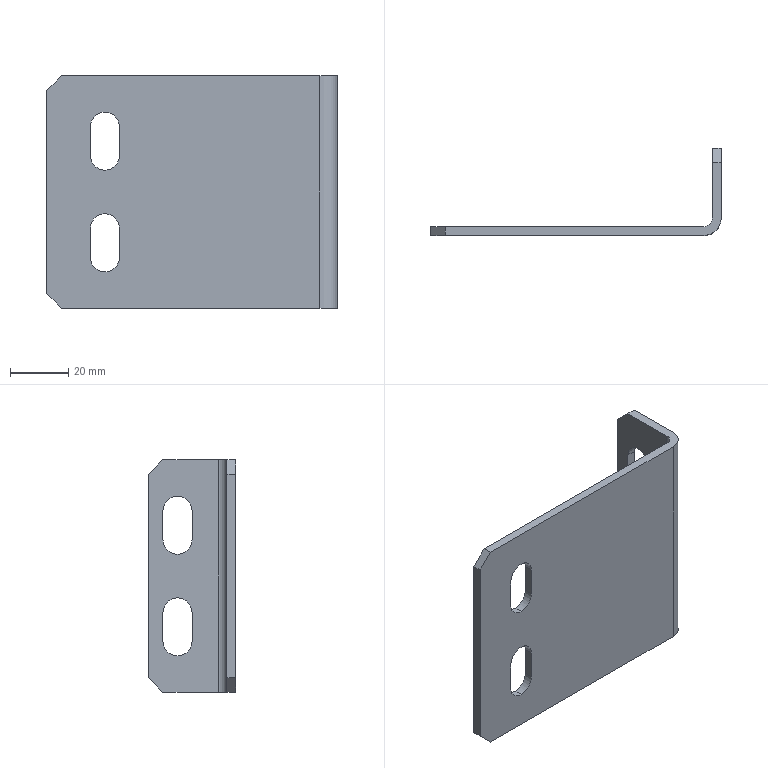Part | STEP file | VD-SYL0380DJ1006_1-9_VD-SYL0380 | 1 solid | 34 faces | box 100 x 30 x 80 mm | volume 27724 mm3 | plane 20 | cylinder 14 | commonest cylinder face diameters 10 x12 6 x1 12 x1
STEP:
#1=CARTESIAN_POINT('',(-75.,3.,-12.5));
#2=VERTEX_POINT('',#1);
#3=CARTESIAN_POINT('',(-85.,3.,-12.5));
#4=VERTEX_POINT('',#3);
#5=CARTESIAN_POINT('',(-80.,3.,-12.5));
#6=DIRECTION('',(0.,-1.,0.));
#7=DIRECTION('',(1.,0.,0.));
#8=AXIS2_PLACEMENT_3D('',#5,#6,#7);
#9=CIRCLE('',#8,5.);
#10=EDGE_CURVE('',#2,#4,#9,.T.);
#11=ORIENTED_EDGE('',*,*,#10,.F.);
#12=CARTESIAN_POINT('',(-75.,0.,-12.5));
#13=VERTEX_POINT('',#12);
#14=CARTESIAN_POINT('',(-75.,3.,-12.5));
#15=DIRECTION('',(0.,-1.,0.));
#16=VECTOR('',#15,1000.);
#17=LINE('',#14,#16);
#18=EDGE_CURVE('',#2,#13,#17,.T.);
#19=ORIENTED_EDGE('',*,*,#18,.T.);
#20=CARTESIAN_POINT('',(-85.,0.,-12.5));
#21=VERTEX_POINT('',#20);
#22=CARTESIAN_POINT('',(-80.,0.,-12.5));
#23=DIRECTION('',(0.,1.,0.));
#24=DIRECTION('',(-1.,0.,0.));
#25=AXIS2_PLACEMENT_3D('',#22,#23,#24);
#26=CIRCLE('',#25,5.);
#27=EDGE_CURVE('',#21,#13,#26,.T.);
#28=ORIENTED_EDGE('',*,*,#27,.F.);
#29=CARTESIAN_POINT('',(-85.,0.,-12.5));
#30=DIRECTION('',(0.,1.,0.));
#31=VECTOR('',#30,1000.);
#32=LINE('',#29,#31);
#33=EDGE_CURVE('',#21,#4,#32,.T.);
#34=ORIENTED_EDGE('',*,*,#33,.T.);
#35=EDGE_LOOP('',(#11,#19,#28,#34));
#36=FACE_OUTER_BOUND('',#35,.T.);
#37=CARTESIAN_POINT('',(-80.,1.5,-12.5));
#38=DIRECTION('',(0.,-1.,0.));
#39=DIRECTION('',(0.,0.,-1.));
#40=AXIS2_PLACEMENT_3D('',#37,#38,#39);
#41=CYLINDRICAL_SURFACE('',#40,5.);
#42=ADVANCED_FACE('',(#36),#41,.F.);
#43=CARTESIAN_POINT('',(-85.,0.,-22.5));
#44=VERTEX_POINT('',#43);
#45=CARTESIAN_POINT('',(-85.,0.,-12.5));
#46=DIRECTION('',(0.,0.,-1.));
#47=VECTOR('',#46,1000.);
#48=LINE('',#45,#47);
#49=EDGE_CURVE('',#21,#44,#48,.T.);
#50=ORIENTED_EDGE('',*,*,#49,.T.);
#51=CARTESIAN_POINT('',(-85.,3.,-22.5));
#52=VERTEX_POINT('',#51);
#53=CARTESIAN_POINT('',(-85.,3.,-22.5));
#54=DIRECTION('',(0.,-1.,0.));
#55=VECTOR('',#54,1000.);
#56=LINE('',#53,#55);
#57=EDGE_CURVE('',#52,#44,#56,.T.);
#58=ORIENTED_EDGE('',*,*,#57,.F.);
#59=CARTESIAN_POINT('',(-85.,3.,-12.5));
#60=DIRECTION('',(0.,0.,-1.));
#61=VECTOR('',#60,1000.);
#62=LINE('',#59,#61);
#63=EDGE_CURVE('',#4,#52,#62,.T.);
#64=ORIENTED_EDGE('',*,*,#63,.F.);
#65=ORIENTED_EDGE('',*,*,#33,.F.);
#66=EDGE_LOOP('',(#50,#58,#64,#65));
#67=FACE_OUTER_BOUND('',#66,.T.);
#68=CARTESIAN_POINT('',(-85.,1.5,-17.5));
#69=DIRECTION('',(1.,0.,0.));
#70=DIRECTION('',(0.,1.,0.));
#71=AXIS2_PLACEMENT_3D('',#68,#69,#70);
#72=PLANE('',#71);
#73=ADVANCED_FACE('',(#67),#72,.T.);
#74=CARTESIAN_POINT('',(-80.,3.,-27.5));
#75=VERTEX_POINT('',#74);
#76=CARTESIAN_POINT('',(-80.,3.,-22.5));
#77=DIRECTION('',(0.,-1.,0.));
#78=DIRECTION('',(-1.,0.,0.));
#79=AXIS2_PLACEMENT_3D('',#76,#77,#78);
#80=CIRCLE('',#79,5.);
#81=EDGE_CURVE('',#52,#75,#80,.T.);
#82=ORIENTED_EDGE('',*,*,#81,.F.);
#83=ORIENTED_EDGE('',*,*,#57,.T.);
#84=CARTESIAN_POINT('',(-80.,0.,-27.5));
#85=VERTEX_POINT('',#84);
#86=CARTESIAN_POINT('',(-80.,0.,-22.5));
#87=DIRECTION('',(0.,1.,0.));
#88=DIRECTION('',(0.,0.,-1.));
#89=AXIS2_PLACEMENT_3D('',#86,#87,#88);
#90=CIRCLE('',#89,5.);
#91=EDGE_CURVE('',#85,#44,#90,.T.);
#92=ORIENTED_EDGE('',*,*,#91,.F.);
#93=CARTESIAN_POINT('',(-80.,0.,-27.5));
#94=DIRECTION('',(0.,1.,0.));
#95=VECTOR('',#94,1000.);
#96=LINE('',#93,#95);
#97=EDGE_CURVE('',#85,#75,#96,.T.);
#98=ORIENTED_EDGE('',*,*,#97,.T.);
#99=EDGE_LOOP('',(#82,#83,#92,#98));
#100=FACE_OUTER_BOUND('',#99,.T.);
#101=CARTESIAN_POINT('',(-80.,1.5,-22.5));
#102=DIRECTION('',(0.,-1.,0.));
#103=DIRECTION('',(0.,0.,-1.));
#104=AXIS2_PLACEMENT_3D('',#101,#102,#103);
#105=CYLINDRICAL_SURFACE('',#104,5.);
#106=ADVANCED_FACE('',(#100),#105,.F.);
#107=ORIENTED_EDGE('',*,*,#97,.F.);
#108=CARTESIAN_POINT('',(-75.,0.,-22.5));
#109=VERTEX_POINT('',#108);
#110=CARTESIAN_POINT('',(-80.,0.,-22.5));
#111=DIRECTION('',(0.,1.,0.));
#112=DIRECTION('',(1.,0.,0.));
#113=AXIS2_PLACEMENT_3D('',#110,#111,#112);
#114=CIRCLE('',#113,5.);
#115=EDGE_CURVE('',#109,#85,#114,.T.);
#116=ORIENTED_EDGE('',*,*,#115,.F.);
#117=CARTESIAN_POINT('',(-75.,3.,-22.5));
#118=VERTEX_POINT('',#117);
#119=CARTESIAN_POINT('',(-75.,0.,-22.5));
#120=DIRECTION('',(0.,1.,0.));
#121=VECTOR('',#120,1000.);
#122=LINE('',#119,#121);
#123=EDGE_CURVE('',#109,#118,#122,.T.);
#124=ORIENTED_EDGE('',*,*,#123,.T.);
#125=CARTESIAN_POINT('',(-80.,3.,-22.5));
#126=DIRECTION('',(0.,-1.,0.));
#127=DIRECTION('',(0.,0.,-1.));
#128=AXIS2_PLACEMENT_3D('',#125,#126,#127);
#129=CIRCLE('',#128,5.);
#130=EDGE_CURVE('',#75,#118,#129,.T.);
#131=ORIENTED_EDGE('',*,*,#130,.F.);
#132=EDGE_LOOP('',(#107,#116,#124,#131));
#133=FACE_OUTER_BOUND('',#132,.T.);
#134=CARTESIAN_POINT('',(-80.,1.5,-22.5));
#135=DIRECTION('',(0.,-1.,0.));
#136=DIRECTION('',(0.,0.,-1.));
#137=AXIS2_PLACEMENT_3D('',#134,#135,#136);
#138=CYLINDRICAL_SURFACE('',#137,5.);
#139=ADVANCED_FACE('',(#133),#138,.F.);
#140=CARTESIAN_POINT('',(-75.,0.,-22.5));
#141=DIRECTION('',(0.,0.,1.));
#142=VECTOR('',#141,1000.);
#143=LINE('',#140,#142);
#144=EDGE_CURVE('',#109,#13,#143,.T.);
#145=ORIENTED_EDGE('',*,*,#144,.T.);
#146=ORIENTED_EDGE('',*,*,#18,.F.);
#147=CARTESIAN_POINT('',(-75.,3.,-22.5));
#148=DIRECTION('',(0.,0.,1.));
#149=VECTOR('',#148,1000.);
#150=LINE('',#147,#149);
#151=EDGE_CURVE('',#118,#2,#150,.T.);
#152=ORIENTED_EDGE('',*,*,#151,.F.);
#153=ORIENTED_EDGE('',*,*,#123,.F.);
#154=EDGE_LOOP('',(#145,#146,#152,#153));
#155=FACE_OUTER_BOUND('',#154,.T.);
#156=CARTESIAN_POINT('',(-75.,1.5,-17.5));
#157=DIRECTION('',(-1.,0.,0.));
#158=DIRECTION('',(0.,0.,1.));
#159=AXIS2_PLACEMENT_3D('',#156,#157,#158);
#160=PLANE('',#159);
#161=ADVANCED_FACE('',(#155),#160,.T.);
#162=CARTESIAN_POINT('',(-85.,0.,22.5));
#163=VERTEX_POINT('',#162);
#164=CARTESIAN_POINT('',(-85.,0.,12.5));
#165=VERTEX_POINT('',#164);
#166=CARTESIAN_POINT('',(-85.,0.,22.5));
#167=DIRECTION('',(0.,0.,-1.));
#168=VECTOR('',#167,1000.);
#169=LINE('',#166,#168);
#170=EDGE_CURVE('',#163,#165,#169,.T.);
#171=ORIENTED_EDGE('',*,*,#170,.T.);
#172=CARTESIAN_POINT('',(-85.,3.,12.5));
#173=VERTEX_POINT('',#172);
#174=CARTESIAN_POINT('',(-85.,3.,12.5));
#175=DIRECTION('',(0.,-1.,0.));
#176=VECTOR('',#175,1000.);
#177=LINE('',#174,#176);
#178=EDGE_CURVE('',#173,#165,#177,.T.);
#179=ORIENTED_EDGE('',*,*,#178,.F.);
#180=CARTESIAN_POINT('',(-85.,3.,22.5));
#181=VERTEX_POINT('',#180);
#182=CARTESIAN_POINT('',(-85.,3.,22.5));
#183=DIRECTION('',(0.,0.,-1.));
#184=VECTOR('',#183,1000.);
#185=LINE('',#182,#184);
#186=EDGE_CURVE('',#181,#173,#185,.T.);
#187=ORIENTED_EDGE('',*,*,#186,.F.);
#188=CARTESIAN_POINT('',(-85.,0.,22.5));
#189=DIRECTION('',(0.,1.,0.));
#190=VECTOR('',#189,1000.);
#191=LINE('',#188,#190);
#192=EDGE_CURVE('',#163,#181,#191,.T.);
#193=ORIENTED_EDGE('',*,*,#192,.F.);
#194=EDGE_LOOP('',(#171,#179,#187,#193));
#195=FACE_OUTER_BOUND('',#194,.T.);
#196=CARTESIAN_POINT('',(-85.,1.5,17.5));
#197=DIRECTION('',(1.,0.,0.));
#198=DIRECTION('',(0.,1.,0.));
#199=AXIS2_PLACEMENT_3D('',#196,#197,#198);
#200=PLANE('',#199);
#201=ADVANCED_FACE('',(#195),#200,.T.);
#202=CARTESIAN_POINT('',(-75.,3.,22.5));
#203=VERTEX_POINT('',#202);
#204=CARTESIAN_POINT('',(-80.,3.,22.5));
#205=DIRECTION('',(0.,-1.,0.));
#206=DIRECTION('',(1.,0.,0.));
#207=AXIS2_PLACEMENT_3D('',#204,#205,#206);
#208=CIRCLE('',#207,5.);
#209=EDGE_CURVE('',#203,#181,#208,.T.);
#210=ORIENTED_EDGE('',*,*,#209,.F.);
#211=CARTESIAN_POINT('',(-75.,0.,22.5));
#212=VERTEX_POINT('',#211);
#213=CARTESIAN_POINT('',(-75.,3.,22.5));
#214=DIRECTION('',(0.,-1.,0.));
#215=VECTOR('',#214,1000.);
#216=LINE('',#213,#215);
#217=EDGE_CURVE('',#203,#212,#216,.T.);
#218=ORIENTED_EDGE('',*,*,#217,.T.);
#219=CARTESIAN_POINT('',(-80.,0.,22.5));
#220=DIRECTION('',(0.,1.,0.));
#221=DIRECTION('',(-1.,0.,0.));
#222=AXIS2_PLACEMENT_3D('',#219,#220,#221);
#223=CIRCLE('',#222,5.);
#224=EDGE_CURVE('',#163,#212,#223,.T.);
#225=ORIENTED_EDGE('',*,*,#224,.F.);
#226=ORIENTED_EDGE('',*,*,#192,.T.);
#227=EDGE_LOOP('',(#210,#218,#225,#226));
#228=FACE_OUTER_BOUND('',#227,.T.);
#229=CARTESIAN_POINT('',(-80.,1.5,22.5));
#230=DIRECTION('',(0.,-1.,0.));
#231=DIRECTION('',(0.,0.,-1.));
#232=AXIS2_PLACEMENT_3D('',#229,#230,#231);
#233=CYLINDRICAL_SURFACE('',#232,5.);
#234=ADVANCED_FACE('',(#228),#233,.F.);
#235=CARTESIAN_POINT('',(-75.,0.,12.5));
#236=VERTEX_POINT('',#235);
#237=CARTESIAN_POINT('',(-75.,0.,12.5));
#238=DIRECTION('',(0.,0.,1.));
#239=VECTOR('',#238,1000.);
#240=LINE('',#237,#239);
#241=EDGE_CURVE('',#236,#212,#240,.T.);
#242=ORIENTED_EDGE('',*,*,#241,.T.);
#243=ORIENTED_EDGE('',*,*,#217,.F.);
#244=CARTESIAN_POINT('',(-75.,3.,12.5));
#245=VERTEX_POINT('',#244);
#246=CARTESIAN_POINT('',(-75.,3.,12.5));
#247=DIRECTION('',(0.,0.,1.));
#248=VECTOR('',#247,1000.);
#249=LINE('',#246,#248);
#250=EDGE_CURVE('',#245,#203,#249,.T.);
#251=ORIENTED_EDGE('',*,*,#250,.F.);
#252=CARTESIAN_POINT('',(-75.,0.,12.5));
#253=DIRECTION('',(0.,1.,0.));
#254=VECTOR('',#253,1000.);
#255=LINE('',#252,#254);
#256=EDGE_CURVE('',#236,#245,#255,.T.);
#257=ORIENTED_EDGE('',*,*,#256,.F.);
#258=EDGE_LOOP('',(#242,#243,#251,#257));
#259=FACE_OUTER_BOUND('',#258,.T.);
#260=CARTESIAN_POINT('',(-75.,1.5,17.5));
#261=DIRECTION('',(-1.,0.,0.));
#262=DIRECTION('',(0.,0.,1.));
#263=AXIS2_PLACEMENT_3D('',#260,#261,#262);
#264=PLANE('',#263);
#265=ADVANCED_FACE('',(#259),#264,.T.);
#266=CARTESIAN_POINT('',(-80.,0.,7.5));
#267=VERTEX_POINT('',#266);
#268=CARTESIAN_POINT('',(-80.,3.,7.5));
#269=VERTEX_POINT('',#268);
#270=CARTESIAN_POINT('',(-80.,0.,7.5));
#271=DIRECTION('',(0.,1.,0.));
#272=VECTOR('',#271,1000.);
#273=LINE('',#270,#272);
#274=EDGE_CURVE('',#267,#269,#273,.T.);
#275=ORIENTED_EDGE('',*,*,#274,.F.);
#276=CARTESIAN_POINT('',(-80.,0.,12.5));
#277=DIRECTION('',(0.,1.,0.));
#278=DIRECTION('',(1.,0.,0.));
#279=AXIS2_PLACEMENT_3D('',#276,#277,#278);
#280=CIRCLE('',#279,5.);
#281=EDGE_CURVE('',#236,#267,#280,.T.);
#282=ORIENTED_EDGE('',*,*,#281,.F.);
#283=ORIENTED_EDGE('',*,*,#256,.T.);
#284=CARTESIAN_POINT('',(-80.,3.,12.5));
#285=DIRECTION('',(0.,-1.,0.));
#286=DIRECTION('',(0.,0.,-1.));
#287=AXIS2_PLACEMENT_3D('',#284,#285,#286);
#288=CIRCLE('',#287,5.);
#289=EDGE_CURVE('',#269,#245,#288,.T.);
#290=ORIENTED_EDGE('',*,*,#289,.F.);
#291=EDGE_LOOP('',(#275,#282,#283,#290));
#292=FACE_OUTER_BOUND('',#291,.T.);
#293=CARTESIAN_POINT('',(-80.,1.5,12.5));
#294=DIRECTION('',(0.,-1.,0.));
#295=DIRECTION('',(0.,0.,-1.));
#296=AXIS2_PLACEMENT_3D('',#293,#294,#295);
#297=CYLINDRICAL_SURFACE('',#296,5.);
#298=ADVANCED_FACE('',(#292),#297,.F.);
#299=CARTESIAN_POINT('',(-80.,3.,12.5));
#300=DIRECTION('',(0.,-1.,0.));
#301=DIRECTION('',(-1.,0.,0.));
#302=AXIS2_PLACEMENT_3D('',#299,#300,#301);
#303=CIRCLE('',#302,5.);
#304=EDGE_CURVE('',#173,#269,#303,.T.);
#305=ORIENTED_EDGE('',*,*,#304,.F.);
#306=ORIENTED_EDGE('',*,*,#178,.T.);
#307=CARTESIAN_POINT('',(-80.,0.,12.5));
#308=DIRECTION('',(0.,1.,0.));
#309=DIRECTION('',(0.,0.,-1.));
#310=AXIS2_PLACEMENT_3D('',#307,#308,#309);
#311=CIRCLE('',#310,5.);
#312=EDGE_CURVE('',#267,#165,#311,.T.);
#313=ORIENTED_EDGE('',*,*,#312,.F.);
#314=ORIENTED_EDGE('',*,*,#274,.T.);
#315=EDGE_LOOP('',(#305,#306,#313,#314));
#316=FACE_OUTER_BOUND('',#315,.T.);
#317=CARTESIAN_POINT('',(-80.,1.5,12.5));
#318=DIRECTION('',(0.,-1.,0.));
#319=DIRECTION('',(0.,0.,-1.));
#320=AXIS2_PLACEMENT_3D('',#317,#318,#319);
#321=CYLINDRICAL_SURFACE('',#320,5.);
#322=ADVANCED_FACE('',(#316),#321,.F.);
#323=CARTESIAN_POINT('',(0.,15.,22.5));
#324=VERTEX_POINT('',#323);
#325=CARTESIAN_POINT('',(0.,20.,27.5));
#326=VERTEX_POINT('',#325);
#327=CARTESIAN_POINT('',(0.,20.,22.5));
#328=DIRECTION('',(-1.,0.,0.));
#329=DIRECTION('',(0.,-1.,0.));
#330=AXIS2_PLACEMENT_3D('',#327,#328,#329);
#331=CIRCLE('',#330,5.);
#332=EDGE_CURVE('',#324,#326,#331,.T.);
#333=ORIENTED_EDGE('',*,*,#332,.F.);
#334=CARTESIAN_POINT('',(-3.,15.,22.5));
#335=VERTEX_POINT('',#334);
#336=CARTESIAN_POINT('',(0.,15.,22.5));
#337=DIRECTION('',(-1.,0.,0.));
#338=VECTOR('',#337,1000.);
#339=LINE('',#336,#338);
#340=EDGE_CURVE('',#324,#335,#339,.T.);
#341=ORIENTED_EDGE('',*,*,#340,.T.);
#342=CARTESIAN_POINT('',(-3.,20.,27.5));
#343=VERTEX_POINT('',#342);
#344=CARTESIAN_POINT('',(-3.,20.,22.5));
#345=DIRECTION('',(1.,0.,0.));
#346=DIRECTION('',(0.,0.,1.));
#347=AXIS2_PLACEMENT_3D('',#344,#345,#346);
#348=CIRCLE('',#347,5.);
#349=EDGE_CURVE('',#343,#335,#348,.T.);
#350=ORIENTED_EDGE('',*,*,#349,.F.);
#351=CARTESIAN_POINT('',(-3.,20.,27.5));
#352=DIRECTION('',(1.,0.,0.));
#353=VECTOR('',#352,1000.);
#354=LINE('',#351,#353);
#355=EDGE_CURVE('',#343,#326,#354,.T.);
#356=ORIENTED_EDGE('',*,*,#355,.T.);
#357=EDGE_LOOP('',(#333,#341,#350,#356));
#358=FACE_OUTER_BOUND('',#357,.T.);
#359=CARTESIAN_POINT('',(-1.5,20.,22.5));
#360=DIRECTION('',(-1.,0.,0.));
#361=DIRECTION('',(0.,0.,1.));
#362=AXIS2_PLACEMENT_3D('',#359,#360,#361);
#363=CYLINDRICAL_SURFACE('',#362,5.);
#364=ADVANCED_FACE('',(#358),#363,.F.);
#365=ORIENTED_EDGE('',*,*,#355,.F.);
#366=CARTESIAN_POINT('',(-3.,25.,22.5));
#367=VERTEX_POINT('',#366);
#368=CARTESIAN_POINT('',(-3.,20.,22.5));
#369=DIRECTION('',(1.,0.,0.));
#370=DIRECTION('',(0.,1.,0.));
#371=AXIS2_PLACEMENT_3D('',#368,#369,#370);
#372=CIRCLE('',#371,5.);
#373=EDGE_CURVE('',#367,#343,#372,.T.);
#374=ORIENTED_EDGE('',*,*,#373,.F.);
#375=CARTESIAN_POINT('',(0.,25.,22.5));
#376=VERTEX_POINT('',#375);
#377=CARTESIAN_POINT('',(-3.,25.,22.5));
#378=DIRECTION('',(1.,0.,0.));
#379=VECTOR('',#378,1000.);
#380=LINE('',#377,#379);
#381=EDGE_CURVE('',#367,#376,#380,.T.);
#382=ORIENTED_EDGE('',*,*,#381,.T.);
#383=CARTESIAN_POINT('',(0.,20.,22.5));
#384=DIRECTION('',(-1.,0.,0.));
#385=DIRECTION('',(0.,0.,1.));
#386=AXIS2_PLACEMENT_3D('',#383,#384,#385);
#387=CIRCLE('',#386,5.);
#388=EDGE_CURVE('',#326,#376,#387,.T.);
#389=ORIENTED_EDGE('',*,*,#388,.F.);
#390=EDGE_LOOP('',(#365,#374,#382,#389));
#391=FACE_OUTER_BOUND('',#390,.T.);
#392=CARTESIAN_POINT('',(-1.5,20.,22.5));
#393=DIRECTION('',(-1.,0.,0.));
#394=DIRECTION('',(0.,0.,1.));
#395=AXIS2_PLACEMENT_3D('',#392,#393,#394);
#396=CYLINDRICAL_SURFACE('',#395,5.);
#397=ADVANCED_FACE('',(#391),#396,.F.);
#398=CARTESIAN_POINT('',(0.,25.,12.5));
#399=VERTEX_POINT('',#398);
#400=CARTESIAN_POINT('',(-3.,25.,12.5));
#401=VERTEX_POINT('',#400);
#402=CARTESIAN_POINT('',(0.,25.,12.5));
#403=DIRECTION('',(-1.,0.,0.));
#404=VECTOR('',#403,1000.);
#405=LINE('',#402,#404);
#406=EDGE_CURVE('',#399,#401,#405,.T.);
#407=ORIENTED_EDGE('',*,*,#406,.F.);
#408=CARTESIAN_POINT('',(0.,25.,12.5));
#409=DIRECTION('',(0.,0.,1.));
#410=VECTOR('',#409,1000.);
#411=LINE('',#408,#410);
#412=EDGE_CURVE('',#399,#376,#411,.T.);
#413=ORIENTED_EDGE('',*,*,#412,.T.);
#414=ORIENTED_EDGE('',*,*,#381,.F.);
#415=CARTESIAN_POINT('',(-3.,25.,22.5));
#416=DIRECTION('',(0.,0.,-1.));
#417=VECTOR('',#416,1000.);
#418=LINE('',#415,#417);
#419=EDGE_CURVE('',#367,#401,#418,.T.);
#420=ORIENTED_EDGE('',*,*,#419,.T.);
#421=EDGE_LOOP('',(#407,#413,#414,#420));
#422=FACE_OUTER_BOUND('',#421,.T.);
#423=CARTESIAN_POINT('',(-1.5,25.,17.5));
#424=DIRECTION('',(0.,1.,0.));
#425=DIRECTION('',(1.,0.,0.));
#426=AXIS2_PLACEMENT_3D('',#423,#424,#425);
#427=PLANE('',#426);
#428=ADVANCED_FACE('',(#422),#427,.F.);
#429=CARTESIAN_POINT('',(-3.,15.,12.5));
#430=VERTEX_POINT('',#429);
#431=CARTESIAN_POINT('',(-3.,20.,12.5));
#432=DIRECTION('',(1.,0.,0.));
#433=DIRECTION('',(0.,0.,-1.));
#434=AXIS2_PLACEMENT_3D('',#431,#432,#433);
#435=CIRCLE('',#434,5.);
#436=EDGE_CURVE('',#430,#401,#435,.T.);
#437=ORIENTED_EDGE('',*,*,#436,.F.);
#438=CARTESIAN_POINT('',(0.,15.,12.5));
#439=VERTEX_POINT('',#438);
#440=CARTESIAN_POINT('',(-3.,15.,12.5));
#441=DIRECTION('',(1.,0.,0.));
#442=VECTOR('',#441,1000.);
#443=LINE('',#440,#442);
#444=EDGE_CURVE('',#430,#439,#443,.T.);
#445=ORIENTED_EDGE('',*,*,#444,.T.);
#446=CARTESIAN_POINT('',(0.,20.,12.5));
#447=DIRECTION('',(-1.,0.,0.));
#448=DIRECTION('',(0.,1.,0.));
#449=AXIS2_PLACEMENT_3D('',#446,#447,#448);
#450=CIRCLE('',#449,5.);
#451=EDGE_CURVE('',#399,#439,#450,.T.);
#452=ORIENTED_EDGE('',*,*,#451,.F.);
#453=ORIENTED_EDGE('',*,*,#406,.T.);
#454=EDGE_LOOP('',(#437,#445,#452,#453));
#455=FACE_OUTER_BOUND('',#454,.T.);
#456=CARTESIAN_POINT('',(-1.5,20.,12.5));
#457=DIRECTION('',(-1.,0.,0.));
#458=DIRECTION('',(0.,0.,1.));
#459=AXIS2_PLACEMENT_3D('',#456,#457,#458);
#460=CYLINDRICAL_SURFACE('',#459,5.);
#461=ADVANCED_FACE('',(#455),#460,.F.);
#462=ORIENTED_EDGE('',*,*,#340,.F.);
#463=CARTESIAN_POINT('',(0.,15.,22.5));
#464=DIRECTION('',(0.,0.,-1.));
#465=VECTOR('',#464,1000.);
#466=LINE('',#463,#465);
#467=EDGE_CURVE('',#324,#439,#466,.T.);
#468=ORIENTED_EDGE('',*,*,#467,.T.);
#469=ORIENTED_EDGE('',*,*,#444,.F.);
#470=CARTESIAN_POINT('',(-3.,15.,12.5));
#471=DIRECTION('',(0.,0.,1.));
#472=VECTOR('',#471,1000.);
#473=LINE('',#470,#472);
#474=EDGE_CURVE('',#430,#335,#473,.T.);
#475=ORIENTED_EDGE('',*,*,#474,.T.);
#476=EDGE_LOOP('',(#462,#468,#469,#475));
#477=FACE_OUTER_BOUND('',#476,.T.);
#478=CARTESIAN_POINT('',(-1.5,15.,17.5));
#479=DIRECTION('',(0.,-1.,0.));
#480=DIRECTION('',(0.,0.,-1.));
#481=AXIS2_PLACEMENT_3D('',#478,#479,#480);
#482=PLANE('',#481);
#483=ADVANCED_FACE('',(#477),#482,.F.);
#484=CARTESIAN_POINT('',(0.,15.,-12.5));
#485=VERTEX_POINT('',#484);
#486=CARTESIAN_POINT('',(-3.,15.,-12.5));
#487=VERTEX_POINT('',#486);
#488=CARTESIAN_POINT('',(0.,15.,-12.5));
#489=DIRECTION('',(-1.,0.,0.));
#490=VECTOR('',#489,1000.);
#491=LINE('',#488,#490);
#492=EDGE_CURVE('',#485,#487,#491,.T.);
#493=ORIENTED_EDGE('',*,*,#492,.F.);
#494=CARTESIAN_POINT('',(0.,15.,-22.5));
#495=VERTEX_POINT('',#494);
#496=CARTESIAN_POINT('',(0.,15.,-12.5));
#497=DIRECTION('',(0.,0.,-1.));
#498=VECTOR('',#497,1000.);
#499=LINE('',#496,#498);
#500=EDGE_CURVE('',#485,#495,#499,.T.);
#501=ORIENTED_EDGE('',*,*,#500,.T.);
#502=CARTESIAN_POINT('',(-3.,15.,-22.5));
#503=VERTEX_POINT('',#502);
#504=CARTESIAN_POINT('',(-3.,15.,-22.5));
#505=DIRECTION('',(1.,0.,0.));
#506=VECTOR('',#505,1000.);
#507=LINE('',#504,#506);
#508=EDGE_CURVE('',#503,#495,#507,.T.);
#509=ORIENTED_EDGE('',*,*,#508,.F.);
#510=CARTESIAN_POINT('',(-3.,15.,-22.5));
#511=DIRECTION('',(0.,0.,1.));
#512=VECTOR('',#511,1000.);
#513=LINE('',#510,#512);
#514=EDGE_CURVE('',#503,#487,#513,.T.);
#515=ORIENTED_EDGE('',*,*,#514,.T.);
#516=EDGE_LOOP('',(#493,#501,#509,#515));
#517=FACE_OUTER_BOUND('',#516,.T.);
#518=CARTESIAN_POINT('',(-1.5,15.,-17.5));
#519=DIRECTION('',(0.,-1.,0.));
#520=DIRECTION('',(0.,0.,-1.));
#521=AXIS2_PLACEMENT_3D('',#518,#519,#520);
#522=PLANE('',#521);
#523=ADVANCED_FACE('',(#517),#522,.F.);
#524=CARTESIAN_POINT('',(-3.,25.,-22.5));
#525=VERTEX_POINT('',#524);
#526=CARTESIAN_POINT('',(-3.,20.,-22.5));
#527=DIRECTION('',(1.,0.,0.));
#528=DIRECTION('',(0.,-1.,0.));
#529=AXIS2_PLACEMENT_3D('',#526,#527,#528);
#530=CIRCLE('',#529,5.);
#531=EDGE_CURVE('',#503,#525,#530,.T.);
#532=ORIENTED_EDGE('',*,*,#531,.F.);
#533=ORIENTED_EDGE('',*,*,#508,.T.);
#534=CARTESIAN_POINT('',(0.,25.,-22.5));
#535=VERTEX_POINT('',#534);
#536=CARTESIAN_POINT('',(0.,20.,-22.5));
#537=DIRECTION('',(-1.,0.,0.));
#538=DIRECTION('',(0.,1.,0.));
#539=AXIS2_PLACEMENT_3D('',#536,#537,#538);
#540=CIRCLE('',#539,5.);
#541=EDGE_CURVE('',#535,#495,#540,.T.);
#542=ORIENTED_EDGE('',*,*,#541,.F.);
#543=CARTESIAN_POINT('',(0.,25.,-22.5));
#544=DIRECTION('',(-1.,0.,0.));
#545=VECTOR('',#544,1000.);
#546=LINE('',#543,#545);
#547=EDGE_CURVE('',#535,#525,#546,.T.);
#548=ORIENTED_EDGE('',*,*,#547,.T.);
#549=EDGE_LOOP('',(#532,#533,#542,#548));
#550=FACE_OUTER_BOUND('',#549,.T.);
#551=CARTESIAN_POINT('',(-1.5,20.,-22.5));
#552=DIRECTION('',(-1.,0.,0.));
#553=DIRECTION('',(0.,0.,1.));
#554=AXIS2_PLACEMENT_3D('',#551,#552,#553);
#555=CYLINDRICAL_SURFACE('',#554,5.);
#556=ADVANCED_FACE('',(#550),#555,.F.);
#557=ORIENTED_EDGE('',*,*,#547,.F.);
#558=CARTESIAN_POINT('',(0.,25.,-12.5));
#559=VERTEX_POINT('',#558);
#560=CARTESIAN_POINT('',(0.,25.,-22.5));
#561=DIRECTION('',(0.,0.,1.));
#562=VECTOR('',#561,1000.);
#563=LINE('',#560,#562);
#564=EDGE_CURVE('',#535,#559,#563,.T.);
#565=ORIENTED_EDGE('',*,*,#564,.T.);
#566=CARTESIAN_POINT('',(-3.,25.,-12.5));
#567=VERTEX_POINT('',#566);
#568=CARTESIAN_POINT('',(-3.,25.,-12.5));
#569=DIRECTION('',(1.,0.,0.));
#570=VECTOR('',#569,1000.);
#571=LINE('',#568,#570);
#572=EDGE_CURVE('',#567,#559,#571,.T.);
#573=ORIENTED_EDGE('',*,*,#572,.F.);
#574=CARTESIAN_POINT('',(-3.,25.,-12.5));
#575=DIRECTION('',(0.,0.,-1.));
#576=VECTOR('',#575,1000.);
#577=LINE('',#574,#576);
#578=EDGE_CURVE('',#567,#525,#577,.T.);
#579=ORIENTED_EDGE('',*,*,#578,.T.);
#580=EDGE_LOOP('',(#557,#565,#573,#579));
#581=FACE_OUTER_BOUND('',#580,.T.);
#582=CARTESIAN_POINT('',(-1.5,25.,-17.5));
#583=DIRECTION('',(0.,1.,0.));
#584=DIRECTION('',(1.,0.,0.));
#585=AXIS2_PLACEMENT_3D('',#582,#583,#584);
#586=PLANE('',#585);
#587=ADVANCED_FACE('',(#581),#586,.F.);
#588=CARTESIAN_POINT('',(-3.,20.,-7.5));
#589=VERTEX_POINT('',#588);
#590=CARTESIAN_POINT('',(0.,20.,-7.5));
#591=VERTEX_POINT('',#590);
#592=CARTESIAN_POINT('',(-3.,20.,-7.5));
#593=DIRECTION('',(1.,0.,0.));
#594=VECTOR('',#593,1000.);
#595=LINE('',#592,#594);
#596=EDGE_CURVE('',#589,#591,#595,.T.);
#597=ORIENTED_EDGE('',*,*,#596,.F.);
#598=CARTESIAN_POINT('',(-3.,20.,-12.5));
#599=DIRECTION('',(1.,0.,0.));
#600=DIRECTION('',(0.,1.,0.));
#601=AXIS2_PLACEMENT_3D('',#598,#599,#600);
#602=CIRCLE('',#601,5.);
#603=EDGE_CURVE('',#567,#589,#602,.T.);
#604=ORIENTED_EDGE('',*,*,#603,.F.);
#605=ORIENTED_EDGE('',*,*,#572,.T.);
#606=CARTESIAN_POINT('',(0.,20.,-12.5));
#607=DIRECTION('',(-1.,0.,0.));
#608=DIRECTION('',(0.,0.,1.));
#609=AXIS2_PLACEMENT_3D('',#606,#607,#608);
#610=CIRCLE('',#609,5.);
#611=EDGE_CURVE('',#591,#559,#610,.T.);
#612=ORIENTED_EDGE('',*,*,#611,.F.);
#613=EDGE_LOOP('',(#597,#604,#605,#612));
#614=FACE_OUTER_BOUND('',#613,.T.);
#615=CARTESIAN_POINT('',(-1.5,20.,-12.5));
#616=DIRECTION('',(-1.,0.,0.));
#617=DIRECTION('',(0.,0.,1.));
#618=AXIS2_PLACEMENT_3D('',#615,#616,#617);
#619=CYLINDRICAL_SURFACE('',#618,5.);
#620=ADVANCED_FACE('',(#614),#619,.F.);
#621=CARTESIAN_POINT('',(0.,20.,-12.5));
#622=DIRECTION('',(-1.,0.,0.));
#623=DIRECTION('',(0.,-1.,0.));
#624=AXIS2_PLACEMENT_3D('',#621,#622,#623);
#625=CIRCLE('',#624,5.);
#626=EDGE_CURVE('',#485,#591,#625,.T.);
#627=ORIENTED_EDGE('',*,*,#626,.F.);
#628=ORIENTED_EDGE('',*,*,#492,.T.);
#629=CARTESIAN_POINT('',(-3.,20.,-12.5));
#630=DIRECTION('',(1.,0.,0.));
#631=DIRECTION('',(0.,0.,1.));
#632=AXIS2_PLACEMENT_3D('',#629,#630,#631);
#633=CIRCLE('',#632,5.);
#634=EDGE_CURVE('',#589,#487,#633,.T.);
#635=ORIENTED_EDGE('',*,*,#634,.F.);
#636=ORIENTED_EDGE('',*,*,#596,.T.);
#637=EDGE_LOOP('',(#627,#628,#635,#636));
#638=FACE_OUTER_BOUND('',#637,.T.);
#639=CARTESIAN_POINT('',(-1.5,20.,-12.5));
#640=DIRECTION('',(-1.,0.,0.));
#641=DIRECTION('',(0.,0.,1.));
#642=AXIS2_PLACEMENT_3D('',#639,#640,#641);
#643=CYLINDRICAL_SURFACE('',#642,5.);
#644=ADVANCED_FACE('',(#638),#643,.F.);
#645=CARTESIAN_POINT('',(0.,30.,35.));
#646=VERTEX_POINT('',#645);
#647=CARTESIAN_POINT('',(0.,25.,40.));
#648=VERTEX_POINT('',#647);
#649=CARTESIAN_POINT('',(0.,30.,35.));
#650=DIRECTION('',(0.,-0.7071,0.7071));
#651=VECTOR('',#650,1000.);
#652=LINE('',#649,#651);
#653=EDGE_CURVE('',#646,#648,#652,.T.);
#654=ORIENTED_EDGE('',*,*,#653,.F.);
#655=CARTESIAN_POINT('',(-3.,30.,35.));
#656=VERTEX_POINT('',#655);
#657=CARTESIAN_POINT('',(-3.,30.,35.));
#658=DIRECTION('',(1.,0.,0.));
#659=VECTOR('',#658,1000.);
#660=LINE('',#657,#659);
#661=EDGE_CURVE('',#656,#646,#660,.T.);
#662=ORIENTED_EDGE('',*,*,#661,.F.);
#663=CARTESIAN_POINT('',(-3.,25.,40.));
#664=VERTEX_POINT('',#663);
#665=CARTESIAN_POINT('',(-3.,25.,40.));
#666=DIRECTION('',(0.,0.7071,-0.7071));
#667=VECTOR('',#666,1000.);
#668=LINE('',#665,#667);
#669=EDGE_CURVE('',#664,#656,#668,.T.);
#670=ORIENTED_EDGE('',*,*,#669,.F.);
#671=CARTESIAN_POINT('',(0.,25.,40.));
#672=DIRECTION('',(-1.,0.,0.));
#673=VECTOR('',#672,1000.);
#674=LINE('',#671,#673);
#675=EDGE_CURVE('',#648,#664,#674,.T.);
#676=ORIENTED_EDGE('',*,*,#675,.F.);
#677=EDGE_LOOP('',(#654,#662,#670,#676));
#678=FACE_OUTER_BOUND('',#677,.T.);
#679=CARTESIAN_POINT('',(-1.5,27.5,37.5));
#680=DIRECTION('',(0.,0.7071,0.7071));
#681=DIRECTION('',(1.,0.,0.));
#682=AXIS2_PLACEMENT_3D('',#679,#680,#681);
#683=PLANE('',#682);
#684=ADVANCED_FACE('',(#678),#683,.T.);
#685=CARTESIAN_POINT('',(-6.,0.,40.));
#686=VERTEX_POINT('',#685);
#687=CARTESIAN_POINT('',(-6.,0.,-40.));
#688=VERTEX_POINT('',#687);
#689=CARTESIAN_POINT('',(-6.,0.,40.));
#690=DIRECTION('',(0.,0.,-1.));
#691=VECTOR('',#690,1000.);
#692=LINE('',#689,#691);
#693=EDGE_CURVE('',#686,#688,#692,.T.);
#694=ORIENTED_EDGE('',*,*,#693,.T.);
#695=CARTESIAN_POINT('',(0.,6.,-40.));
#696=VERTEX_POINT('',#695);
#697=CARTESIAN_POINT('',(-6.,6.,-40.));
#698=DIRECTION('',(0.,0.,-1.));
#699=DIRECTION('',(1.,0.,0.));
#700=AXIS2_PLACEMENT_3D('',#697,#698,#699);
#701=CIRCLE('',#700,6.);
#702=EDGE_CURVE('',#696,#688,#701,.T.);
#703=ORIENTED_EDGE('',*,*,#702,.F.);
#704=CARTESIAN_POINT('',(0.,6.,40.));
#705=VERTEX_POINT('',#704);
#706=CARTESIAN_POINT('',(0.,6.,-40.));
#707=DIRECTION('',(0.,0.,1.));
#708=VECTOR('',#707,1000.);
#709=LINE('',#706,#708);
#710=EDGE_CURVE('',#696,#705,#709,.T.);
#711=ORIENTED_EDGE('',*,*,#710,.T.);
#712=CARTESIAN_POINT('',(-6.,6.,40.));
#713=DIRECTION('',(0.,0.,1.));
#714=DIRECTION('',(0.,-1.,0.));
#715=AXIS2_PLACEMENT_3D('',#712,#713,#714);
#716=CIRCLE('',#715,6.);
#717=EDGE_CURVE('',#686,#705,#716,.T.);
#718=ORIENTED_EDGE('',*,*,#717,.F.);
#719=EDGE_LOOP('',(#694,#703,#711,#718));
#720=FACE_OUTER_BOUND('',#719,.T.);
#721=CARTESIAN_POINT('',(-6.,6.,144.288));
#722=DIRECTION('',(0.,0.,-1.));
#723=DIRECTION('',(-1.,0.,0.));
#724=AXIS2_PLACEMENT_3D('',#721,#722,#723);
#725=CYLINDRICAL_SURFACE('',#724,6.);
#726=ADVANCED_FACE('',(#720),#725,.T.);
#727=ORIENTED_EDGE('',*,*,#332,.T.);
#728=ORIENTED_EDGE('',*,*,#388,.T.);
#729=ORIENTED_EDGE('',*,*,#412,.F.);
#730=ORIENTED_EDGE('',*,*,#451,.T.);
#731=ORIENTED_EDGE('',*,*,#467,.F.);
#732=EDGE_LOOP('',(#727,#728,#729,#730,#731));
#733=FACE_BOUND('',#732,.T.);
#734=ORIENTED_EDGE('',*,*,#611,.T.);
#735=ORIENTED_EDGE('',*,*,#564,.F.);
#736=ORIENTED_EDGE('',*,*,#541,.T.);
#737=ORIENTED_EDGE('',*,*,#500,.F.);
#738=ORIENTED_EDGE('',*,*,#626,.T.);
#739=EDGE_LOOP('',(#734,#735,#736,#737,#738));
#740=FACE_BOUND('',#739,.T.);
#741=CARTESIAN_POINT('',(0.,25.,-40.));
#742=VERTEX_POINT('',#741);
#743=CARTESIAN_POINT('',(0.,30.,-35.));
#744=VERTEX_POINT('',#743);
#745=CARTESIAN_POINT('',(0.,25.,-40.));
#746=DIRECTION('',(0.,0.7071,0.7071));
#747=VECTOR('',#746,1000.);
#748=LINE('',#745,#747);
#749=EDGE_CURVE('',#742,#744,#748,.T.);
#750=ORIENTED_EDGE('',*,*,#749,.T.);
#751=CARTESIAN_POINT('',(0.,30.,35.));
#752=DIRECTION('',(0.,0.,-1.));
#753=VECTOR('',#752,1000.);
#754=LINE('',#751,#753);
#755=EDGE_CURVE('',#646,#744,#754,.T.);
#756=ORIENTED_EDGE('',*,*,#755,.F.);
#757=ORIENTED_EDGE('',*,*,#653,.T.);
#758=CARTESIAN_POINT('',(0.,6.,40.));
#759=DIRECTION('',(0.,1.,0.));
#760=VECTOR('',#759,1000.);
#761=LINE('',#758,#760);
#762=EDGE_CURVE('',#705,#648,#761,.T.);
#763=ORIENTED_EDGE('',*,*,#762,.F.);
#764=ORIENTED_EDGE('',*,*,#710,.F.);
#765=CARTESIAN_POINT('',(0.,25.,-40.));
#766=DIRECTION('',(0.,-1.,0.));
#767=VECTOR('',#766,1000.);
#768=LINE('',#765,#767);
#769=EDGE_CURVE('',#742,#696,#768,.T.);
#770=ORIENTED_EDGE('',*,*,#769,.F.);
#771=EDGE_LOOP('',(#750,#756,#757,#763,#764,#770));
#772=FACE_OUTER_BOUND('',#771,.T.);
#773=CARTESIAN_POINT('',(0.,0.,-40.));
#774=DIRECTION('',(1.,0.,0.));
#775=DIRECTION('',(0.,1.,0.));
#776=AXIS2_PLACEMENT_3D('',#773,#774,#775);
#777=PLANE('',#776);
#778=ADVANCED_FACE('',(#733,#740,#772),#777,.T.);
#779=CARTESIAN_POINT('',(-3.,30.,-35.));
#780=VERTEX_POINT('',#779);
#781=CARTESIAN_POINT('',(0.,30.,-35.));
#782=DIRECTION('',(-1.,0.,0.));
#783=VECTOR('',#782,1000.);
#784=LINE('',#781,#783);
#785=EDGE_CURVE('',#744,#780,#784,.T.);
#786=ORIENTED_EDGE('',*,*,#785,.T.);
#787=CARTESIAN_POINT('',(-3.,30.,35.));
#788=DIRECTION('',(0.,0.,-1.));
#789=VECTOR('',#788,1000.);
#790=LINE('',#787,#789);
#791=EDGE_CURVE('',#656,#780,#790,.T.);
#792=ORIENTED_EDGE('',*,*,#791,.F.);
#793=ORIENTED_EDGE('',*,*,#661,.T.);
#794=ORIENTED_EDGE('',*,*,#755,.T.);
#795=EDGE_LOOP('',(#786,#792,#793,#794));
#796=FACE_OUTER_BOUND('',#795,.T.);
#797=CARTESIAN_POINT('',(-1.5,30.,0.));
#798=DIRECTION('',(0.,1.,0.));
#799=DIRECTION('',(1.,0.,0.));
#800=AXIS2_PLACEMENT_3D('',#797,#798,#799);
#801=PLANE('',#800);
#802=ADVANCED_FACE('',(#796),#801,.T.);
#803=ORIENTED_EDGE('',*,*,#749,.F.);
#804=CARTESIAN_POINT('',(-3.,25.,-40.));
#805=VERTEX_POINT('',#804);
#806=CARTESIAN_POINT('',(-3.,25.,-40.));
#807=DIRECTION('',(1.,0.,0.));
#808=VECTOR('',#807,1000.);
#809=LINE('',#806,#808);
#810=EDGE_CURVE('',#805,#742,#809,.T.);
#811=ORIENTED_EDGE('',*,*,#810,.F.);
#812=CARTESIAN_POINT('',(-3.,30.,-35.));
#813=DIRECTION('',(0.,-0.7071,-0.7071));
#814=VECTOR('',#813,1000.);
#815=LINE('',#812,#814);
#816=EDGE_CURVE('',#780,#805,#815,.T.);
#817=ORIENTED_EDGE('',*,*,#816,.F.);
#818=ORIENTED_EDGE('',*,*,#785,.F.);
#819=EDGE_LOOP('',(#803,#811,#817,#818));
#820=FACE_OUTER_BOUND('',#819,.T.);
#821=CARTESIAN_POINT('',(-1.5,27.5,-37.5));
#822=DIRECTION('',(0.,0.7071,-0.7071));
#823=DIRECTION('',(-1.,0.,0.));
#824=AXIS2_PLACEMENT_3D('',#821,#822,#823);
#825=PLANE('',#824);
#826=ADVANCED_FACE('',(#820),#825,.T.);
#827=ORIENTED_EDGE('',*,*,#531,.T.);
#828=ORIENTED_EDGE('',*,*,#578,.F.);
#829=ORIENTED_EDGE('',*,*,#603,.T.);
#830=ORIENTED_EDGE('',*,*,#634,.T.);
#831=ORIENTED_EDGE('',*,*,#514,.F.);
#832=EDGE_LOOP('',(#827,#828,#829,#830,#831));
#833=FACE_BOUND('',#832,.T.);
#834=ORIENTED_EDGE('',*,*,#436,.T.);
#835=ORIENTED_EDGE('',*,*,#419,.F.);
#836=ORIENTED_EDGE('',*,*,#373,.T.);
#837=ORIENTED_EDGE('',*,*,#349,.T.);
#838=ORIENTED_EDGE('',*,*,#474,.F.);
#839=EDGE_LOOP('',(#834,#835,#836,#837,#838));
#840=FACE_BOUND('',#839,.T.);
#841=CARTESIAN_POINT('',(-3.,6.,40.));
#842=VERTEX_POINT('',#841);
#843=CARTESIAN_POINT('',(-3.,25.,40.));
#844=DIRECTION('',(0.,-1.,0.));
#845=VECTOR('',#844,1000.);
#846=LINE('',#843,#845);
#847=EDGE_CURVE('',#664,#842,#846,.T.);
#848=ORIENTED_EDGE('',*,*,#847,.F.);
#849=ORIENTED_EDGE('',*,*,#669,.T.);
#850=ORIENTED_EDGE('',*,*,#791,.T.);
#851=ORIENTED_EDGE('',*,*,#816,.T.);
#852=CARTESIAN_POINT('',(-3.,6.,-40.));
#853=VERTEX_POINT('',#852);
#854=CARTESIAN_POINT('',(-3.,25.,-40.));
#855=DIRECTION('',(0.,-1.,0.));
#856=VECTOR('',#855,1000.);
#857=LINE('',#854,#856);
#858=EDGE_CURVE('',#805,#853,#857,.T.);
#859=ORIENTED_EDGE('',*,*,#858,.T.);
#860=CARTESIAN_POINT('',(-3.,6.,40.));
#861=DIRECTION('',(0.,0.,-1.));
#862=VECTOR('',#861,1000.);
#863=LINE('',#860,#862);
#864=EDGE_CURVE('',#842,#853,#863,.T.);
#865=ORIENTED_EDGE('',*,*,#864,.F.);
#866=EDGE_LOOP('',(#848,#849,#850,#851,#859,#865));
#867=FACE_OUTER_BOUND('',#866,.T.);
#868=CARTESIAN_POINT('',(-3.,0.,-40.));
#869=DIRECTION('',(1.,0.,0.));
#870=DIRECTION('',(0.,1.,0.));
#871=AXIS2_PLACEMENT_3D('',#868,#869,#870);
#872=PLANE('',#871);
#873=ADVANCED_FACE('',(#833,#840,#867),#872,.F.);
#874=CARTESIAN_POINT('',(-6.,3.,-40.));
#875=VERTEX_POINT('',#874);
#876=CARTESIAN_POINT('',(-6.,6.,-40.));
#877=DIRECTION('',(0.,0.,1.));
#878=DIRECTION('',(0.,-1.,0.));
#879=AXIS2_PLACEMENT_3D('',#876,#877,#878);
#880=CIRCLE('',#879,3.);
#881=EDGE_CURVE('',#875,#853,#880,.T.);
#882=ORIENTED_EDGE('',*,*,#881,.F.);
#883=CARTESIAN_POINT('',(-6.,3.,40.));
#884=VERTEX_POINT('',#883);
#885=CARTESIAN_POINT('',(-6.,3.,-40.));
#886=DIRECTION('',(0.,0.,1.));
#887=VECTOR('',#886,1000.);
#888=LINE('',#885,#887);
#889=EDGE_CURVE('',#875,#884,#888,.T.);
#890=ORIENTED_EDGE('',*,*,#889,.T.);
#891=CARTESIAN_POINT('',(-6.,6.,40.));
#892=DIRECTION('',(0.,0.,-1.));
#893=DIRECTION('',(1.,0.,0.));
#894=AXIS2_PLACEMENT_3D('',#891,#892,#893);
#895=CIRCLE('',#894,3.);
#896=EDGE_CURVE('',#842,#884,#895,.T.);
#897=ORIENTED_EDGE('',*,*,#896,.F.);
#898=ORIENTED_EDGE('',*,*,#864,.T.);
#899=EDGE_LOOP('',(#882,#890,#897,#898));
#900=FACE_OUTER_BOUND('',#899,.T.);
#901=CARTESIAN_POINT('',(-6.,6.,144.288));
#902=DIRECTION('',(0.,0.,-1.));
#903=DIRECTION('',(-1.,0.,0.));
#904=AXIS2_PLACEMENT_3D('',#901,#902,#903);
#905=CYLINDRICAL_SURFACE('',#904,3.);
#906=ADVANCED_FACE('',(#900),#905,.F.);
#907=ORIENTED_EDGE('',*,*,#10,.T.);
#908=ORIENTED_EDGE('',*,*,#63,.T.);
#909=ORIENTED_EDGE('',*,*,#81,.T.);
#910=ORIENTED_EDGE('',*,*,#130,.T.);
#911=ORIENTED_EDGE('',*,*,#151,.T.);
#912=EDGE_LOOP('',(#907,#908,#909,#910,#911));
#913=FACE_BOUND('',#912,.T.);
#914=ORIENTED_EDGE('',*,*,#289,.T.);
#915=ORIENTED_EDGE('',*,*,#250,.T.);
#916=ORIENTED_EDGE('',*,*,#209,.T.);
#917=ORIENTED_EDGE('',*,*,#186,.T.);
#918=ORIENTED_EDGE('',*,*,#304,.T.);
#919=EDGE_LOOP('',(#914,#915,#916,#917,#918));
#920=FACE_BOUND('',#919,.T.);
#921=CARTESIAN_POINT('',(-95.,3.,-40.));
#922=VERTEX_POINT('',#921);
#923=CARTESIAN_POINT('',(-6.,3.,-40.));
#924=DIRECTION('',(-1.,0.,0.));
#925=VECTOR('',#924,1000.);
#926=LINE('',#923,#925);
#927=EDGE_CURVE('',#875,#922,#926,.T.);
#928=ORIENTED_EDGE('',*,*,#927,.T.);
#929=CARTESIAN_POINT('',(-100.,3.,-35.));
#930=VERTEX_POINT('',#929);
#931=CARTESIAN_POINT('',(-95.,3.,-40.));
#932=DIRECTION('',(-0.7071,0.,0.7071));
#933=VECTOR('',#932,1000.);
#934=LINE('',#931,#933);
#935=EDGE_CURVE('',#922,#930,#934,.T.);
#936=ORIENTED_EDGE('',*,*,#935,.T.);
#937=CARTESIAN_POINT('',(-100.,3.,35.));
#938=VERTEX_POINT('',#937);
#939=CARTESIAN_POINT('',(-100.,3.,35.));
#940=DIRECTION('',(0.,0.,-1.));
#941=VECTOR('',#940,1000.);
#942=LINE('',#939,#941);
#943=EDGE_CURVE('',#938,#930,#942,.T.);
#944=ORIENTED_EDGE('',*,*,#943,.F.);
#945=CARTESIAN_POINT('',(-95.,3.,40.));
#946=VERTEX_POINT('',#945);
#947=CARTESIAN_POINT('',(-100.,3.,35.));
#948=DIRECTION('',(0.7071,0.,0.7071));
#949=VECTOR('',#948,1000.);
#950=LINE('',#947,#949);
#951=EDGE_CURVE('',#938,#946,#950,.T.);
#952=ORIENTED_EDGE('',*,*,#951,.T.);
#953=CARTESIAN_POINT('',(-6.,3.,40.));
#954=DIRECTION('',(-1.,0.,0.));
#955=VECTOR('',#954,1000.);
#956=LINE('',#953,#955);
#957=EDGE_CURVE('',#884,#946,#956,.T.);
#958=ORIENTED_EDGE('',*,*,#957,.F.);
#959=ORIENTED_EDGE('',*,*,#889,.F.);
#960=EDGE_LOOP('',(#928,#936,#944,#952,#958,#959));
#961=FACE_OUTER_BOUND('',#960,.T.);
#962=CARTESIAN_POINT('',(-100.,3.,-40.));
#963=DIRECTION('',(0.,-1.,0.));
#964=DIRECTION('',(0.,0.,-1.));
#965=AXIS2_PLACEMENT_3D('',#962,#963,#964);
#966=PLANE('',#965);
#967=ADVANCED_FACE('',(#913,#920,#961),#966,.F.);
#968=CARTESIAN_POINT('',(-100.,0.,-35.));
#969=VERTEX_POINT('',#968);
#970=CARTESIAN_POINT('',(-95.,0.,-40.));
#971=VERTEX_POINT('',#970);
#972=CARTESIAN_POINT('',(-100.,0.,-35.));
#973=DIRECTION('',(0.7071,0.,-0.7071));
#974=VECTOR('',#973,1000.);
#975=LINE('',#972,#974);
#976=EDGE_CURVE('',#969,#971,#975,.T.);
#977=ORIENTED_EDGE('',*,*,#976,.F.);
#978=CARTESIAN_POINT('',(-100.,3.,-35.));
#979=DIRECTION('',(0.,-1.,0.));
#980=VECTOR('',#979,1000.);
#981=LINE('',#978,#980);
#982=EDGE_CURVE('',#930,#969,#981,.T.);
#983=ORIENTED_EDGE('',*,*,#982,.F.);
#984=ORIENTED_EDGE('',*,*,#935,.F.);
#985=CARTESIAN_POINT('',(-95.,3.,-40.));
#986=DIRECTION('',(0.,-1.,0.));
#987=VECTOR('',#986,1000.);
#988=LINE('',#985,#987);
#989=EDGE_CURVE('',#922,#971,#988,.T.);
#990=ORIENTED_EDGE('',*,*,#989,.T.);
#991=EDGE_LOOP('',(#977,#983,#984,#990));
#992=FACE_OUTER_BOUND('',#991,.T.);
#993=CARTESIAN_POINT('',(-97.5,1.5,-37.5));
#994=DIRECTION('',(-0.7071,0.,-0.7071));
#995=DIRECTION('',(-0.7071,0.,0.7071));
#996=AXIS2_PLACEMENT_3D('',#993,#994,#995);
#997=PLANE('',#996);
#998=ADVANCED_FACE('',(#992),#997,.T.);
#999=CARTESIAN_POINT('',(-100.,0.,35.));
#1000=VERTEX_POINT('',#999);
#1001=CARTESIAN_POINT('',(-100.,0.,-35.));
#1002=DIRECTION('',(0.,0.,1.));
#1003=VECTOR('',#1002,1000.);
#1004=LINE('',#1001,#1003);
#1005=EDGE_CURVE('',#969,#1000,#1004,.T.);
#1006=ORIENTED_EDGE('',*,*,#1005,.T.);
#1007=CARTESIAN_POINT('',(-100.,0.,35.));
#1008=DIRECTION('',(0.,1.,0.));
#1009=VECTOR('',#1008,1000.);
#1010=LINE('',#1007,#1009);
#1011=EDGE_CURVE('',#1000,#938,#1010,.T.);
#1012=ORIENTED_EDGE('',*,*,#1011,.T.);
#1013=ORIENTED_EDGE('',*,*,#943,.T.);
#1014=ORIENTED_EDGE('',*,*,#982,.T.);
#1015=EDGE_LOOP('',(#1006,#1012,#1013,#1014));
#1016=FACE_OUTER_BOUND('',#1015,.T.);
#1017=CARTESIAN_POINT('',(-100.,1.5,0.));
#1018=DIRECTION('',(1.,0.,0.));
#1019=DIRECTION('',(0.,1.,0.));
#1020=AXIS2_PLACEMENT_3D('',#1017,#1018,#1019);
#1021=PLANE('',#1020);
#1022=ADVANCED_FACE('',(#1016),#1021,.F.);
#1023=CARTESIAN_POINT('',(-95.,0.,40.));
#1024=VERTEX_POINT('',#1023);
#1025=CARTESIAN_POINT('',(-95.,0.,40.));
#1026=DIRECTION('',(-0.7071,0.,-0.7071));
#1027=VECTOR('',#1026,1000.);
#1028=LINE('',#1025,#1027);
#1029=EDGE_CURVE('',#1024,#1000,#1028,.T.);
#1030=ORIENTED_EDGE('',*,*,#1029,.F.);
#1031=CARTESIAN_POINT('',(-95.,3.,40.));
#1032=DIRECTION('',(0.,-1.,0.));
#1033=VECTOR('',#1032,1000.);
#1034=LINE('',#1031,#1033);
#1035=EDGE_CURVE('',#946,#1024,#1034,.T.);
#1036=ORIENTED_EDGE('',*,*,#1035,.F.);
#1037=ORIENTED_EDGE('',*,*,#951,.F.);
#1038=ORIENTED_EDGE('',*,*,#1011,.F.);
#1039=EDGE_LOOP('',(#1030,#1036,#1037,#1038));
#1040=FACE_OUTER_BOUND('',#1039,.T.);
#1041=CARTESIAN_POINT('',(-97.5,1.5,37.5));
#1042=DIRECTION('',(-0.7071,0.,0.7071));
#1043=DIRECTION('',(0.,1.,0.));
#1044=AXIS2_PLACEMENT_3D('',#1041,#1042,#1043);
#1045=PLANE('',#1044);
#1046=ADVANCED_FACE('',(#1040),#1045,.T.);
#1047=ORIENTED_EDGE('',*,*,#717,.T.);
#1048=ORIENTED_EDGE('',*,*,#762,.T.);
#1049=ORIENTED_EDGE('',*,*,#675,.T.);
#1050=ORIENTED_EDGE('',*,*,#847,.T.);
#1051=ORIENTED_EDGE('',*,*,#896,.T.);
#1052=ORIENTED_EDGE('',*,*,#957,.T.);
#1053=ORIENTED_EDGE('',*,*,#1035,.T.);
#1054=CARTESIAN_POINT('',(-95.,0.,40.));
#1055=DIRECTION('',(1.,0.,0.));
#1056=VECTOR('',#1055,1000.);
#1057=LINE('',#1054,#1056);
#1058=EDGE_CURVE('',#1024,#686,#1057,.T.);
#1059=ORIENTED_EDGE('',*,*,#1058,.T.);
#1060=EDGE_LOOP('',(#1047,#1048,#1049,#1050,#1051,#1052,#1053,#1059));
#1061=FACE_OUTER_BOUND('',#1060,.T.);
#1062=CARTESIAN_POINT('',(-50.75,1.5,40.));
#1063=DIRECTION('',(0.,0.,-1.));
#1064=DIRECTION('',(0.,-1.,0.));
#1065=AXIS2_PLACEMENT_3D('',#1062,#1063,#1064);
#1066=PLANE('',#1065);
#1067=ADVANCED_FACE('',(#1061),#1066,.F.);
#1068=ORIENTED_EDGE('',*,*,#224,.T.);
#1069=ORIENTED_EDGE('',*,*,#241,.F.);
#1070=ORIENTED_EDGE('',*,*,#281,.T.);
#1071=ORIENTED_EDGE('',*,*,#312,.T.);
#1072=ORIENTED_EDGE('',*,*,#170,.F.);
#1073=EDGE_LOOP('',(#1068,#1069,#1070,#1071,#1072));
#1074=FACE_BOUND('',#1073,.T.);
#1075=ORIENTED_EDGE('',*,*,#91,.T.);
#1076=ORIENTED_EDGE('',*,*,#49,.F.);
#1077=ORIENTED_EDGE('',*,*,#27,.T.);
#1078=ORIENTED_EDGE('',*,*,#144,.F.);
#1079=ORIENTED_EDGE('',*,*,#115,.T.);
#1080=EDGE_LOOP('',(#1075,#1076,#1077,#1078,#1079));
#1081=FACE_BOUND('',#1080,.T.);
#1082=ORIENTED_EDGE('',*,*,#1029,.T.);
#1083=ORIENTED_EDGE('',*,*,#1005,.F.);
#1084=ORIENTED_EDGE('',*,*,#976,.T.);
#1085=CARTESIAN_POINT('',(-6.,0.,-40.));
#1086=DIRECTION('',(-1.,0.,0.));
#1087=VECTOR('',#1086,1000.);
#1088=LINE('',#1085,#1087);
#1089=EDGE_CURVE('',#688,#971,#1088,.T.);
#1090=ORIENTED_EDGE('',*,*,#1089,.F.);
#1091=ORIENTED_EDGE('',*,*,#693,.F.);
#1092=ORIENTED_EDGE('',*,*,#1058,.F.);
#1093=EDGE_LOOP('',(#1082,#1083,#1084,#1090,#1091,#1092));
#1094=FACE_OUTER_BOUND('',#1093,.T.);
#1095=CARTESIAN_POINT('',(-100.,0.,-40.));
#1096=DIRECTION('',(0.,-1.,0.));
#1097=DIRECTION('',(0.,0.,-1.));
#1098=AXIS2_PLACEMENT_3D('',#1095,#1096,#1097);
#1099=PLANE('',#1098);
#1100=ADVANCED_FACE('',(#1074,#1081,#1094),#1099,.T.);
#1101=ORIENTED_EDGE('',*,*,#989,.F.);
#1102=ORIENTED_EDGE('',*,*,#927,.F.);
#1103=ORIENTED_EDGE('',*,*,#881,.T.);
#1104=ORIENTED_EDGE('',*,*,#858,.F.);
#1105=ORIENTED_EDGE('',*,*,#810,.T.);
#1106=ORIENTED_EDGE('',*,*,#769,.T.);
#1107=ORIENTED_EDGE('',*,*,#702,.T.);
#1108=ORIENTED_EDGE('',*,*,#1089,.T.);
#1109=EDGE_LOOP('',(#1101,#1102,#1103,#1104,#1105,#1106,#1107,#1108));
#1110=FACE_OUTER_BOUND('',#1109,.T.);
#1111=CARTESIAN_POINT('',(-50.75,1.5,-40.));
#1112=DIRECTION('',(0.,0.,-1.));
#1113=DIRECTION('',(0.,-1.,0.));
#1114=AXIS2_PLACEMENT_3D('',#1111,#1112,#1113);
#1115=PLANE('',#1114);
#1116=ADVANCED_FACE('',(#1110),#1115,.T.);
#1117=CLOSED_SHELL('',(#42,#73,#106,#139,#161,#201,#234,#265,#298,#322,#364,#397,#428,#461,#483,#523,#556,#587,#620,#644,#684,#726,#778,#802,#826,#873,#906,#967,#998,#1022,#1046,#1067,#1100,#1116));
#1118=MANIFOLD_SOLID_BREP('',#1117);
#1119=CARTESIAN_POINT('',(0.,0.,0.));
#1120=DIRECTION('',(0.,0.,1.));
#1121=DIRECTION('',(1.,0.,0.));
#1122=AXIS2_PLACEMENT_3D('',#1119,#1120,#1121);
#1123=(LENGTH_UNIT()NAMED_UNIT(*)SI_UNIT(.MILLI.,.METRE.));
#1124=UNCERTAINTY_MEASURE_WITH_UNIT(LENGTH_MEASURE(0.00001),#1123,'','');
#1125=(NAMED_UNIT(*)PLANE_ANGLE_UNIT()SI_UNIT($,.RADIAN.));
#1126=(NAMED_UNIT(*)SI_UNIT($,.STERADIAN.)SOLID_ANGLE_UNIT());
#1127=(GEOMETRIC_REPRESENTATION_CONTEXT(3)GLOBAL_UNCERTAINTY_ASSIGNED_CONTEXT((#1124))GLOBAL_UNIT_ASSIGNED_CONTEXT((#1123,#1125,#1126))REPRESENTATION_CONTEXT('',''));
#1128=ADVANCED_BREP_SHAPE_REPRESENTATION('',(#1118,#1122),#1127);